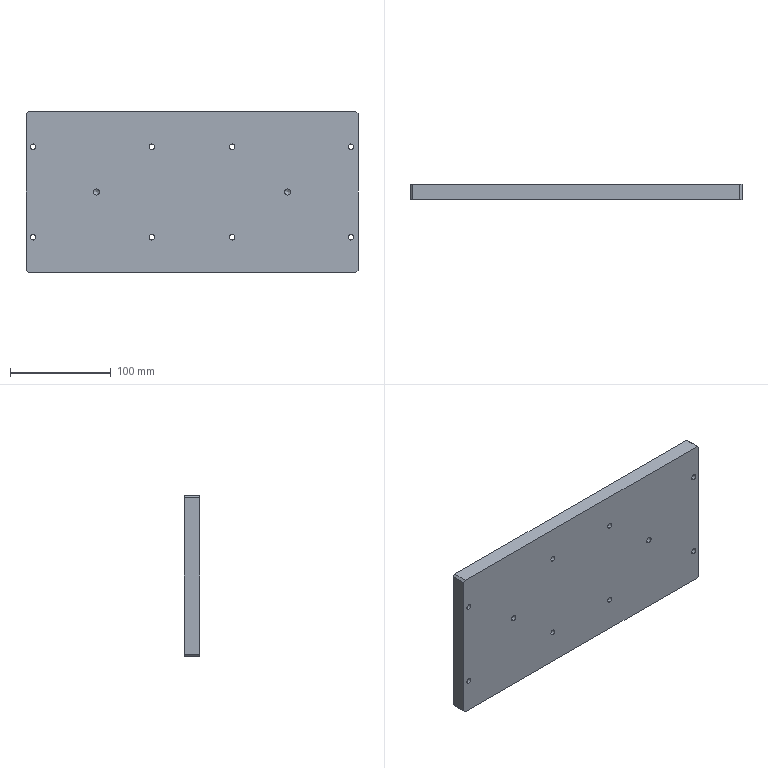Part | SolidWorks | features BaseBody 1 | 1 solid | 58 faces | box 330 x 15 x 160 mm | volume 784405 mm3 | cylinder 36 | plane 18 | cone 4 | commonest cylinder face diameters 5.5 x16 10 x16 6 x4